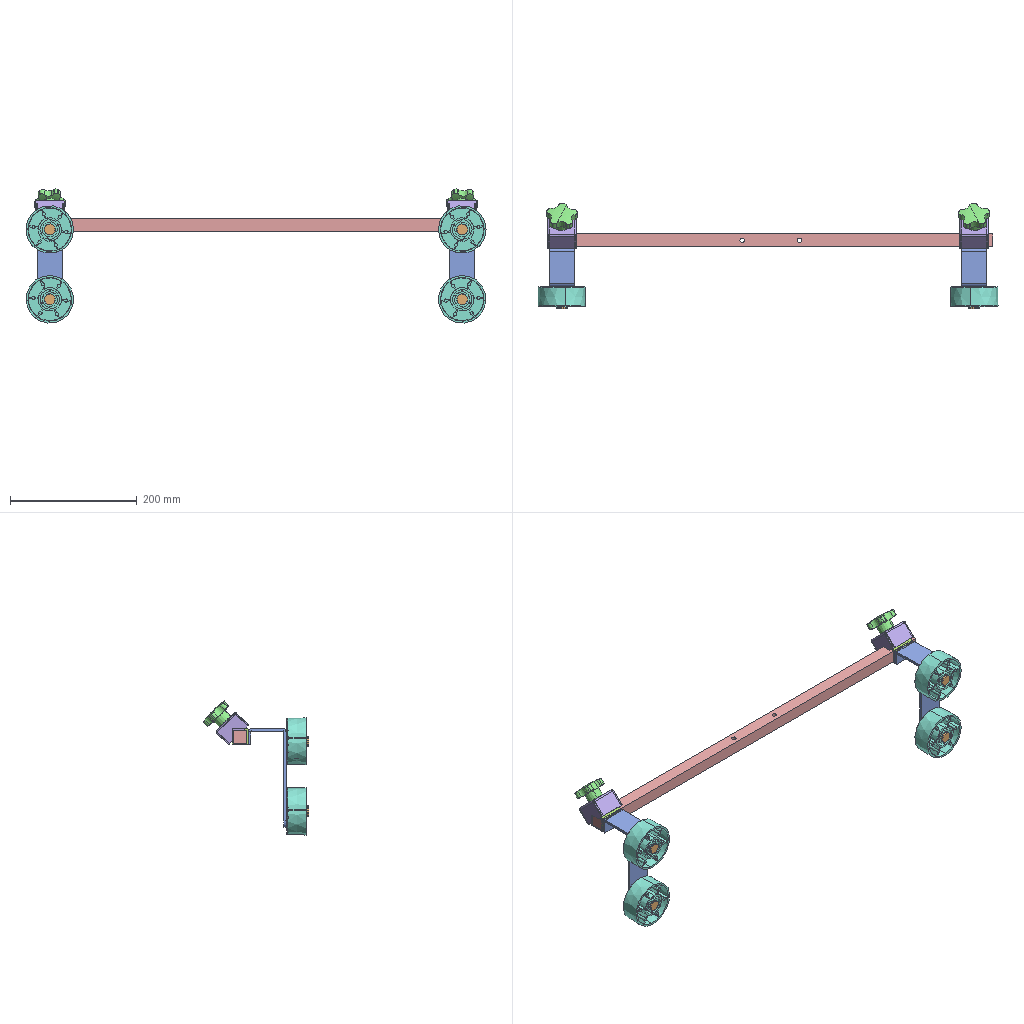Assembly | SolidWorks | 9 different items | 21 placed | box 725 x 166 x 211 mm
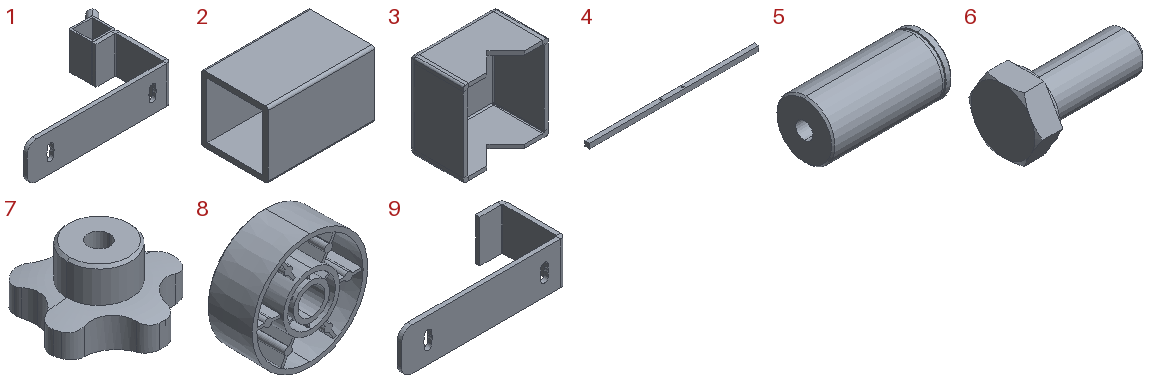Parts list (item | name | quantity | parent item | size | volume | features):
1 | (subassembly) | x2 | - | 179.597 x 109.597 x 40 mm | 46355 mm3 | -
2 | - | x2 | in 1 | 40 x 25 x 25 mm | 7326 mm3 | features BreakCorner 1, FlatPattern 1, SMBaseFlange 1, SheetMetal 1
3 | - | x2 | - | 45 x 29 x 45 mm | 12461 mm3 | features SMWeldBead 4, EdgeFlange 1, FlatPattern 1, ICE 1, SMBaseFlange 1, SheetMetal 1
4 | - | x1 | - | 700 x 20 x 20 mm | 278461 mm3 | features Extrusion 1, ICE 1
5 | - | x4 | - | 35 x 17 x 17 mm | 7604 mm3 | features Chamfer 1, Extrusion 1, HoleWzd 1, RevCut 1
6 | - | x2 | in 1 | 31.4 x 18.475 x 16 mm | 3346 mm3 | features RevCut 4, Chamfer 1, Extrusion 1, Fillet 1, LPattern 1, Revolution 1
7 | - | x2 | - | 48.607 x 46.741 x 26.101 mm | 21839 mm3 | features Chamfer 1, CirPattern 1, Fillet 1, HoleWzd 1, ICE 1, Revolution 1
8 | - | x4 | - | 75 x 31 x 75 mm | 50473 mm3 | features ICE 14, Rib 6, HoleWzd 2, BaseBody 1, Chamfer 1
9 | - | x2 | in 1 | 155 x 60 x 40 mm | 35684 mm3 | features ICE 2, Fillet 1, FlatPattern 1, SMBaseFlange 1, SheetMetal 1
Mates (type | each side: item.copy, entity, surface, feature):
In the top assembly
Width | 2.1 face plane Base-Flange 1 | 2.1 face plane Base-Flange 1 | 4.1 face plane Boss-Extrude 1 | 4.1 face plane Boss-Extrude 1 | 2 times
Concentric | 9.1 face cylinder Cut-Extrude 2 | 8.1 face cylinder M16 HexUnnamedBoltUnnamedCountersunkHole 1
Concentric | 9.1 face cylinder Cut-Extrude 2 | 8.2 face cylinder M16 HexUnnamedBoltUnnamedCountersunkHole 1
Concentric | 8.1 face cylinder M16 HexUnnamedBoltUnnamedCountersunkHole 1 | 5.1 face cylinder Boss-Extrude 1
Coincident | 8.1 face plane Boss-Extrude 14 | 5.1 face plane Cut-Revolve 1
Coincident | 9.1 face plane Base-Flange 1 | 5.1 face plane Boss-Extrude 1
Concentric | 8.2 face cone Input3 | 5.2 face cylinder Boss-Extrude 1
Coincident | 9.1 face plane Base-Flange 1 | 5.2 face plane Boss-Extrude 1
Coincident | 8.2 face plane Boss-Extrude 14 | 5.2 face plane Cut-Revolve 1
Concentric | 6.1 face cylinder Boss-Revolve 1 | 3.1 face cylinder Base-Flange 1
Width | 3.1 face plane Edge-Flange 1 | 3.1 face plane Edge-Flange 1 | 9.1 face plane Base-Flange 1 | 9.1 face plane Base-Flange 1
Coincident | 4.1 face plane Boss-Extrude 1 | 3.1 face plane Cut-Extrude 1
Concentric | 6.1 face cylinder Boss-Revolve 1 | 7.1 face cylinder Revolve 1
Coincident | 3.1 face plane Base-Flange 1 | 7.1 face plane Revolve 1
In subassembly 1
Width | 9.2 face plane Base-Flange 1 | 9.2 face plane Base-Flange 1 | 6.2 face plane Base-Extrude | 6.2 face plane Base-Extrude
Coincident | 2.2 plane | 6.2 plane
Coincident | 9.2 face plane Base-Flange 1 | 2.2 face plane Base-Flange 1 | 3 times
Tangent | 2.2 face cylinder Break-Corner1 | 6.2 face plane Base-Extrude